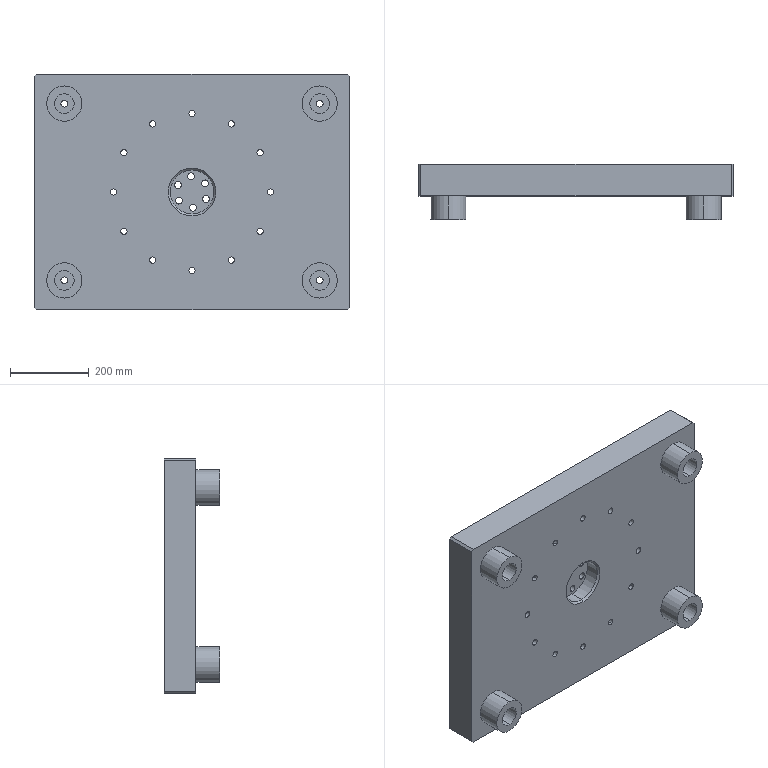Part | SolidWorks | features ICE 3, Chamfer 2, HoleWzd 2, CirPattern 1, Extrusion 1 | 1 solid | 113 faces | box 800 x 140 x 600 mm | volume 38677043 mm3 | cylinder 82 | plane 29 | cone 2 | commonest cylinder face diameters 16 x24 17.5 x20 26 x20 50 x8 90 x8 112 x2